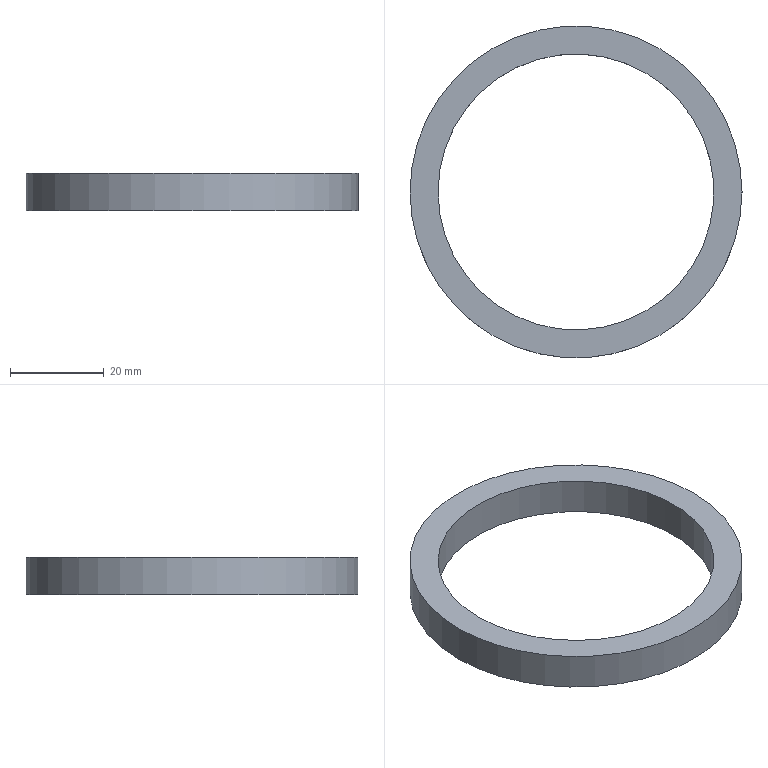Part | STEP file | BRONZE-BUSH2_id534_x_t | 1 solid | 4 faces | box 71 x 71 x 8 mm | volume 9802 mm3 | plane 2 | cylinder 2 | commonest cylinder face diameters 59 x1 71 x1
STEP:
#1=CARTESIAN_POINT('',(-59.5,0.,123.003));
#2=VERTEX_POINT('',#1);
#3=CARTESIAN_POINT('',(-30.,0.,123.003));
#4=DIRECTION('',(0.,0.,-1.));
#5=DIRECTION('',(-1.,0.,0.));
#6=AXIS2_PLACEMENT_3D('',#3,#4,#5);
#7=CIRCLE('',#6,29.5);
#8=EDGE_CURVE('',#2,#2,#7,.T.);
#9=ORIENTED_EDGE('',*,*,#8,.T.);
#10=EDGE_LOOP('',(#9));
#11=FACE_BOUND('',#10,.T.);
#12=CARTESIAN_POINT('',(-65.5,0.,123.003));
#13=VERTEX_POINT('',#12);
#14=CARTESIAN_POINT('',(-30.,0.,123.003));
#15=DIRECTION('',(0.,0.,-1.));
#16=DIRECTION('',(-1.,0.,0.));
#17=AXIS2_PLACEMENT_3D('',#14,#15,#16);
#18=CIRCLE('',#17,35.5);
#19=EDGE_CURVE('',#13,#13,#18,.T.);
#20=ORIENTED_EDGE('',*,*,#19,.F.);
#21=EDGE_LOOP('',(#20));
#22=FACE_BOUND('',#21,.T.);
#23=CARTESIAN_POINT('',(-30.,0.,123.003));
#24=DIRECTION('',(0.,0.,-1.));
#25=DIRECTION('',(-1.,0.,0.));
#26=AXIS2_PLACEMENT_3D('',#23,#24,#25);
#27=PLANE('',#26);
#28=ADVANCED_FACE('',(#11,#22),#27,.F.);
#29=CARTESIAN_POINT('',(-65.5,0.,115.003));
#30=VERTEX_POINT('',#29);
#31=CARTESIAN_POINT('',(-30.,0.,115.003));
#32=DIRECTION('',(0.,0.,-1.));
#33=DIRECTION('',(-1.,0.,0.));
#34=AXIS2_PLACEMENT_3D('',#31,#32,#33);
#35=CIRCLE('',#34,35.5);
#36=EDGE_CURVE('',#30,#30,#35,.T.);
#37=ORIENTED_EDGE('',*,*,#36,.F.);
#38=EDGE_LOOP('',(#37));
#39=FACE_BOUND('',#38,.T.);
#40=ORIENTED_EDGE('',*,*,#19,.T.);
#41=EDGE_LOOP('',(#40));
#42=FACE_BOUND('',#41,.T.);
#43=CARTESIAN_POINT('',(-30.,0.,125.053));
#44=DIRECTION('',(0.,0.,-1.));
#45=DIRECTION('',(-1.,0.,0.));
#46=AXIS2_PLACEMENT_3D('',#43,#44,#45);
#47=CYLINDRICAL_SURFACE('',#46,35.5);
#48=ADVANCED_FACE('',(#39,#42),#47,.T.);
#49=CARTESIAN_POINT('',(-59.5,0.,115.003));
#50=VERTEX_POINT('',#49);
#51=CARTESIAN_POINT('',(-30.,0.,115.003));
#52=DIRECTION('',(0.,0.,1.));
#53=DIRECTION('',(-1.,0.,0.));
#54=AXIS2_PLACEMENT_3D('',#51,#52,#53);
#55=CIRCLE('',#54,29.5);
#56=EDGE_CURVE('',#50,#50,#55,.T.);
#57=ORIENTED_EDGE('',*,*,#56,.F.);
#58=EDGE_LOOP('',(#57));
#59=FACE_BOUND('',#58,.T.);
#60=ORIENTED_EDGE('',*,*,#8,.F.);
#61=EDGE_LOOP('',(#60));
#62=FACE_BOUND('',#61,.T.);
#63=CARTESIAN_POINT('',(-30.,0.,125.053));
#64=DIRECTION('',(0.,0.,-1.));
#65=DIRECTION('',(-1.,0.,0.));
#66=AXIS2_PLACEMENT_3D('',#63,#64,#65);
#67=CYLINDRICAL_SURFACE('',#66,29.5);
#68=ADVANCED_FACE('',(#59,#62),#67,.F.);
#69=ORIENTED_EDGE('',*,*,#56,.T.);
#70=EDGE_LOOP('',(#69));
#71=FACE_BOUND('',#70,.T.);
#72=ORIENTED_EDGE('',*,*,#36,.T.);
#73=EDGE_LOOP('',(#72));
#74=FACE_BOUND('',#73,.T.);
#75=CARTESIAN_POINT('',(-30.,0.,115.003));
#76=DIRECTION('',(0.,0.,-1.));
#77=DIRECTION('',(-1.,0.,0.));
#78=AXIS2_PLACEMENT_3D('',#75,#76,#77);
#79=PLANE('',#78);
#80=ADVANCED_FACE('',(#71,#74),#79,.T.);
#81=CLOSED_SHELL('',(#28,#48,#68,#80));
#82=MANIFOLD_SOLID_BREP('',#81);
#83=(LENGTH_UNIT()NAMED_UNIT(*)SI_UNIT(.MILLI.,.METRE.));
#84=UNCERTAINTY_MEASURE_WITH_UNIT(LENGTH_MEASURE(0.00002),#83,'','');
#85=(NAMED_UNIT(*)PLANE_ANGLE_UNIT()SI_UNIT($,.RADIAN.));
#86=PLANE_ANGLE_MEASURE_WITH_UNIT(PLANE_ANGLE_MEASURE(0.01745),#85);
#87=DIMENSIONAL_EXPONENTS(0.,0.,0.,0.,0.,0.,0.);
#88=(CONVERSION_BASED_UNIT('DEGREE',#86)NAMED_UNIT(#87)PLANE_ANGLE_UNIT());
#89=(NAMED_UNIT(*)SI_UNIT($,.STERADIAN.)SOLID_ANGLE_UNIT());
#90=(GEOMETRIC_REPRESENTATION_CONTEXT(3)GLOBAL_UNCERTAINTY_ASSIGNED_CONTEXT((#84))GLOBAL_UNIT_ASSIGNED_CONTEXT((#83,#88,#89))REPRESENTATION_CONTEXT('',''));
#91=ADVANCED_BREP_SHAPE_REPRESENTATION('',(#82),#90);